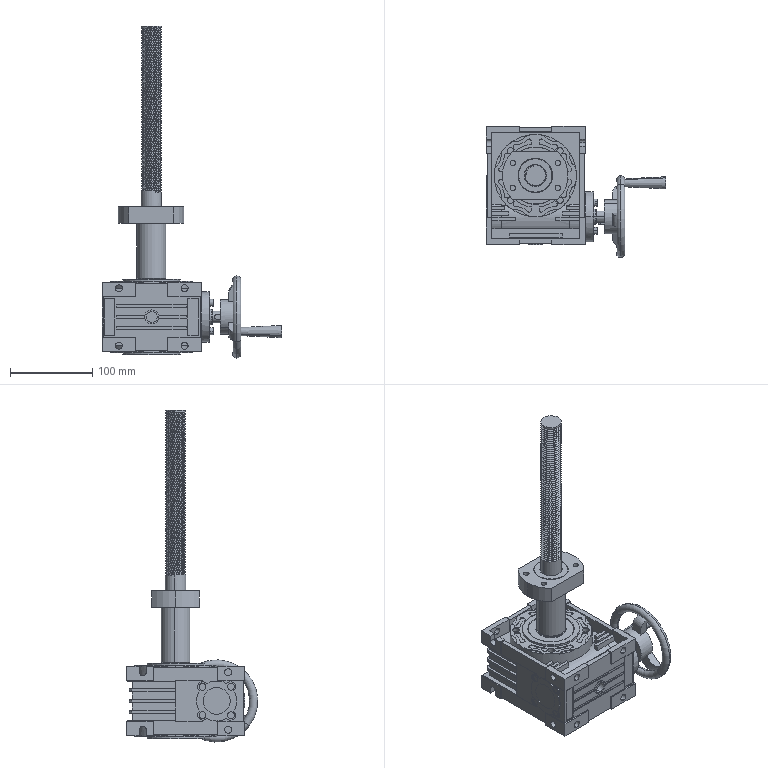Part | SolidWorks | 7 solids | 999 faces | box 219 x 160 x 404 mm | volume 1526813 mm3 | plane 430 | cylinder 415 | torus 87 | cone 32 | sphere 32 | spline 3 | commonest cylinder face diameters 25 x145 4.802 x40 8.5 x36 38.734 x20 57.4 x18 8 x17